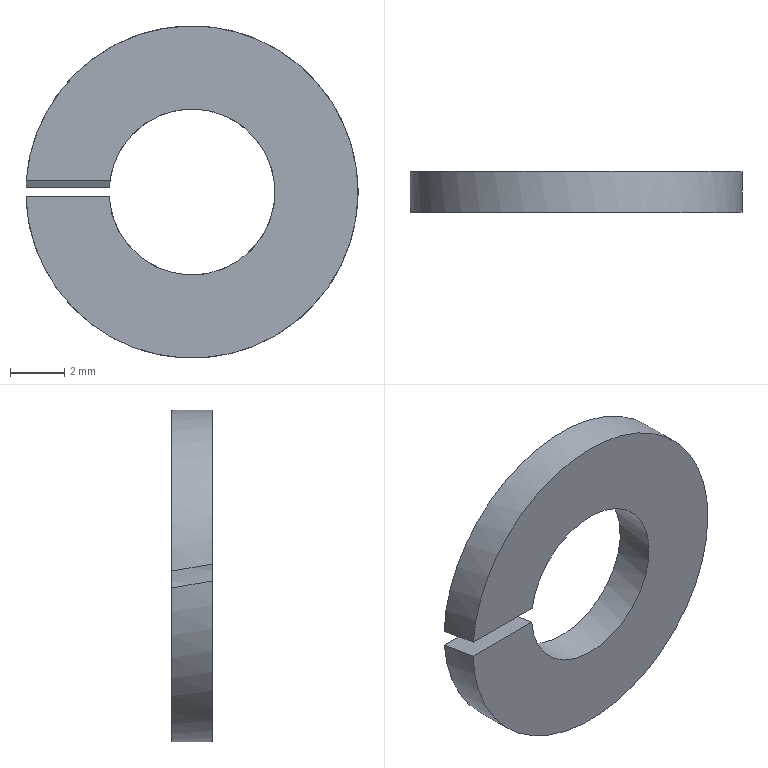Part | NX | features 5003_302_SLW6 2 | 1 solid | 6 faces | box 12.197 x 1.5 x 12.2 mm | volume 128.672 mm3 | plane 4 | cylinder 2 | commonest cylinder face diameters 6.1 x1 12.2 x1
STEP:
#1=CARTESIAN_POINT('',(159.728,0.,-39.32));
#2=VERTEX_POINT('',#1);
#3=CARTESIAN_POINT('',(162.78,0.,-39.32));
#4=VERTEX_POINT('',#3);
#5=CARTESIAN_POINT('',(159.725,0.,-39.32));
#6=DIRECTION('',(1.,0.,0.));
#7=VECTOR('',#6,1000.);
#8=LINE('',#5,#7);
#9=EDGE_CURVE('',#2,#4,#8,.T.);
#10=ORIENTED_EDGE('',*,*,#9,.F.);
#11=CARTESIAN_POINT('',(159.741,0.,-39.94));
#12=VERTEX_POINT('',#11);
#13=CARTESIAN_POINT('',(165.825,0.,-39.5));
#14=DIRECTION('',(0.,1.,0.));
#15=DIRECTION('',(-1.,0.,0.));
#16=AXIS2_PLACEMENT_3D('',#13,#14,#15);
#17=CIRCLE('',#16,6.1);
#18=EDGE_CURVE('',#2,#12,#17,.T.);
#19=ORIENTED_EDGE('',*,*,#18,.T.);
#20=CARTESIAN_POINT('',(162.807,0.,-39.94));
#21=VERTEX_POINT('',#20);
#22=CARTESIAN_POINT('',(159.725,0.,-39.94));
#23=DIRECTION('',(1.,0.,0.));
#24=VECTOR('',#23,1000.);
#25=LINE('',#22,#24);
#26=EDGE_CURVE('',#12,#21,#25,.T.);
#27=ORIENTED_EDGE('',*,*,#26,.T.);
#28=CARTESIAN_POINT('',(165.825,0.,-39.5));
#29=DIRECTION('',(0.,1.,0.));
#30=DIRECTION('',(-1.,0.,0.));
#31=AXIS2_PLACEMENT_3D('',#28,#29,#30);
#32=CIRCLE('',#31,3.05);
#33=EDGE_CURVE('',#4,#21,#32,.T.);
#34=ORIENTED_EDGE('',*,*,#33,.F.);
#35=EDGE_LOOP('',(#10,#19,#27,#34));
#36=FACE_BOUND('',#35,.T.);
#37=CARTESIAN_POINT('',(165.825,0.,-36.45));
#38=DIRECTION('',(0.,-1.,0.));
#39=DIRECTION('',(1.,0.,0.));
#40=AXIS2_PLACEMENT_3D('',#37,#38,#39);
#41=PLANE('',#40);
#42=ADVANCED_FACE('',(#36),#41,.F.);
#43=CARTESIAN_POINT('',(159.741,-1.5,-39.06));
#44=VERTEX_POINT('',#43);
#45=CARTESIAN_POINT('',(165.825,1.038,-39.5));
#46=DIRECTION('',(0.,-0.1708,-0.9853));
#47=DIRECTION('',(0.,0.9853,-0.1708));
#48=AXIS2_PLACEMENT_3D('',#45,#46,#47);
#49=ELLIPSE('',#48,35.717,6.1);
#50=EDGE_CURVE('',#44,#2,#49,.T.);
#51=ORIENTED_EDGE('',*,*,#50,.F.);
#52=CARTESIAN_POINT('',(159.728,-1.5,-39.68));
#53=VERTEX_POINT('',#52);
#54=CARTESIAN_POINT('',(165.825,-1.5,-39.5));
#55=DIRECTION('',(0.,1.,0.));
#56=DIRECTION('',(-1.,0.,0.));
#57=AXIS2_PLACEMENT_3D('',#54,#55,#56);
#58=CIRCLE('',#57,6.1);
#59=EDGE_CURVE('',#44,#53,#58,.T.);
#60=ORIENTED_EDGE('',*,*,#59,.T.);
#61=CARTESIAN_POINT('',(165.825,-2.538,-39.5));
#62=DIRECTION('',(0.,0.1708,0.9853));
#63=DIRECTION('',(0.,0.9853,-0.1708));
#64=AXIS2_PLACEMENT_3D('',#61,#62,#63);
#65=ELLIPSE('',#64,35.717,6.1);
#66=EDGE_CURVE('',#12,#53,#65,.T.);
#67=ORIENTED_EDGE('',*,*,#66,.F.);
#68=ORIENTED_EDGE('',*,*,#18,.F.);
#69=EDGE_LOOP('',(#51,#60,#67,#68));
#70=FACE_BOUND('',#69,.T.);
#71=CARTESIAN_POINT('',(165.825,0.,-39.5));
#72=DIRECTION('',(0.,1.,0.));
#73=DIRECTION('',(-1.,0.,0.));
#74=AXIS2_PLACEMENT_3D('',#71,#72,#73);
#75=CYLINDRICAL_SURFACE('',#74,6.1);
#76=ADVANCED_FACE('',(#70),#75,.T.);
#77=CARTESIAN_POINT('',(162.807,-1.5,-39.06));
#78=VERTEX_POINT('',#77);
#79=CARTESIAN_POINT('',(159.725,-1.5,-39.06));
#80=DIRECTION('',(1.,0.,0.));
#81=VECTOR('',#80,1000.);
#82=LINE('',#79,#81);
#83=EDGE_CURVE('',#44,#78,#82,.T.);
#84=ORIENTED_EDGE('',*,*,#83,.T.);
#85=CARTESIAN_POINT('',(162.78,-1.5,-39.68));
#86=VERTEX_POINT('',#85);
#87=CARTESIAN_POINT('',(165.825,-1.5,-39.5));
#88=DIRECTION('',(0.,1.,0.));
#89=DIRECTION('',(-1.,0.,0.));
#90=AXIS2_PLACEMENT_3D('',#87,#88,#89);
#91=CIRCLE('',#90,3.05);
#92=EDGE_CURVE('',#78,#86,#91,.T.);
#93=ORIENTED_EDGE('',*,*,#92,.T.);
#94=CARTESIAN_POINT('',(159.725,-1.5,-39.68));
#95=DIRECTION('',(1.,0.,0.));
#96=VECTOR('',#95,1000.);
#97=LINE('',#94,#96);
#98=EDGE_CURVE('',#53,#86,#97,.T.);
#99=ORIENTED_EDGE('',*,*,#98,.F.);
#100=ORIENTED_EDGE('',*,*,#59,.F.);
#101=EDGE_LOOP('',(#84,#93,#99,#100));
#102=FACE_BOUND('',#101,.T.);
#103=CARTESIAN_POINT('',(165.825,-1.5,-36.45));
#104=DIRECTION('',(0.,1.,0.));
#105=DIRECTION('',(-1.,0.,0.));
#106=AXIS2_PLACEMENT_3D('',#103,#104,#105);
#107=PLANE('',#106);
#108=ADVANCED_FACE('',(#102),#107,.F.);
#109=CARTESIAN_POINT('',(165.825,1.038,-39.5));
#110=DIRECTION('',(0.,-0.1708,-0.9853));
#111=DIRECTION('',(0.,0.9853,-0.1708));
#112=AXIS2_PLACEMENT_3D('',#109,#110,#111);
#113=ELLIPSE('',#112,17.859,3.05);
#114=EDGE_CURVE('',#4,#78,#113,.F.);
#115=ORIENTED_EDGE('',*,*,#114,.F.);
#116=ORIENTED_EDGE('',*,*,#33,.T.);
#117=CARTESIAN_POINT('',(165.825,-2.538,-39.5));
#118=DIRECTION('',(0.,0.1708,0.9853));
#119=DIRECTION('',(0.,0.9853,-0.1708));
#120=AXIS2_PLACEMENT_3D('',#117,#118,#119);
#121=ELLIPSE('',#120,17.859,3.05);
#122=EDGE_CURVE('',#86,#21,#121,.F.);
#123=ORIENTED_EDGE('',*,*,#122,.F.);
#124=ORIENTED_EDGE('',*,*,#92,.F.);
#125=EDGE_LOOP('',(#115,#116,#123,#124));
#126=FACE_BOUND('',#125,.T.);
#127=CARTESIAN_POINT('',(165.825,0.,-39.5));
#128=DIRECTION('',(0.,1.,0.));
#129=DIRECTION('',(-1.,0.,0.));
#130=AXIS2_PLACEMENT_3D('',#127,#128,#129);
#131=CYLINDRICAL_SURFACE('',#130,3.05);
#132=ADVANCED_FACE('',(#126),#131,.F.);
#133=ORIENTED_EDGE('',*,*,#66,.T.);
#134=ORIENTED_EDGE('',*,*,#98,.T.);
#135=ORIENTED_EDGE('',*,*,#122,.T.);
#136=ORIENTED_EDGE('',*,*,#26,.F.);
#137=EDGE_LOOP('',(#133,#134,#135,#136));
#138=FACE_BOUND('',#137,.T.);
#139=CARTESIAN_POINT('',(159.725,0.,-39.94));
#140=DIRECTION('',(0.,0.1708,0.9853));
#141=DIRECTION('',(0.,0.9853,-0.1708));
#142=AXIS2_PLACEMENT_3D('',#139,#140,#141);
#143=PLANE('',#142);
#144=ADVANCED_FACE('',(#138),#143,.T.);
#145=ORIENTED_EDGE('',*,*,#50,.T.);
#146=ORIENTED_EDGE('',*,*,#9,.T.);
#147=ORIENTED_EDGE('',*,*,#114,.T.);
#148=ORIENTED_EDGE('',*,*,#83,.F.);
#149=EDGE_LOOP('',(#145,#146,#147,#148));
#150=FACE_BOUND('',#149,.T.);
#151=CARTESIAN_POINT('',(159.725,-1.5,-39.06));
#152=DIRECTION('',(0.,-0.1708,-0.9853));
#153=DIRECTION('',(0.,-0.9853,0.1708));
#154=AXIS2_PLACEMENT_3D('',#151,#152,#153);
#155=PLANE('',#154);
#156=ADVANCED_FACE('',(#150),#155,.T.);
#157=CLOSED_SHELL('',(#42,#76,#108,#132,#144,#156));
#158=MANIFOLD_SOLID_BREP('',#157);
#159=(LENGTH_UNIT()NAMED_UNIT(*)SI_UNIT(.MILLI.,.METRE.));
#160=UNCERTAINTY_MEASURE_WITH_UNIT(LENGTH_MEASURE(0.00001),#159,'','');
#161=(NAMED_UNIT(*)PLANE_ANGLE_UNIT()SI_UNIT($,.RADIAN.));
#162=(NAMED_UNIT(*)SI_UNIT($,.STERADIAN.)SOLID_ANGLE_UNIT());
#163=(GEOMETRIC_REPRESENTATION_CONTEXT(3)GLOBAL_UNCERTAINTY_ASSIGNED_CONTEXT((#160))GLOBAL_UNIT_ASSIGNED_CONTEXT((#159,#161,#162))REPRESENTATION_CONTEXT('',''));
#164=ADVANCED_BREP_SHAPE_REPRESENTATION('',(#158),#163);